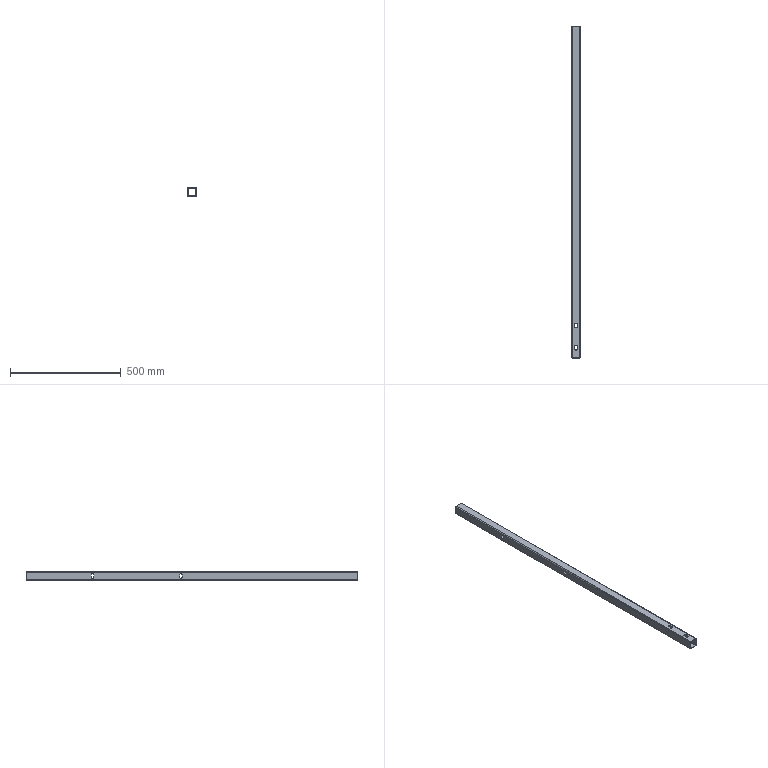Part | STEP file | E3-中转釜护栏2立柱主体_Default<As Machined> | 1 solid | 54 faces | box 40 x 1500 x 40 mm | volume 436819 mm3 | cylinder 28 | plane 26 | commonest cylinder face diameters 12 x20 4 x4 8 x4